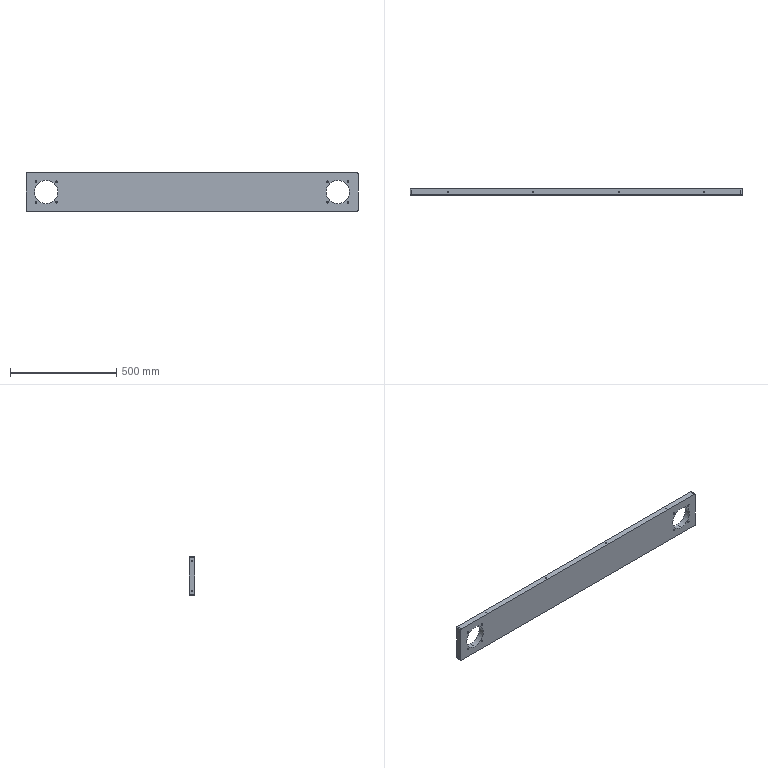Part | SolidWorks | features BaseBody 1 | 1 solid | 62 faces | box 1560 x 28 x 180 mm | volume 7309619 mm3 | cylinder 40 | cone 16 | plane 6 | commonest cylinder face diameters 5 x16 8.5 x16 10 x4 110.5 x4